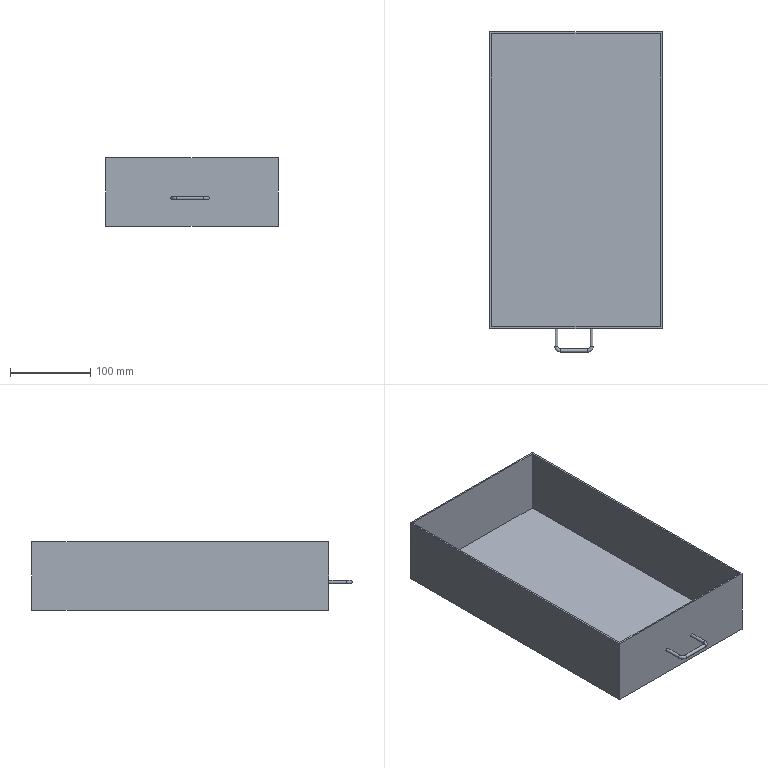Part | NX | features solid 2 | 1 solid | 16 faces | box 215 x 399 x 85 mm | volume 439303 mm3 | plane 11 | cylinder 3 | torus 2 | commonest cylinder face diameters 4 x3
STEP:
#1=CARTESIAN_POINT('',(143.,-305.,-247.));
#2=VERTEX_POINT('',#1);
#3=CARTESIAN_POINT('',(143.,-305.,-245.));
#4=DIRECTION('',(0.,-1.,0.));
#5=DIRECTION('',(0.,0.,-1.));
#6=AXIS2_PLACEMENT_3D('',#3,#4,#5);
#7=CIRCLE('',#6,2.);
#8=EDGE_CURVE('',#2,#2,#7,.F.);
#9=ORIENTED_EDGE('',*,*,#8,.T.);
#10=EDGE_LOOP('',(#9));
#11=FACE_BOUND('',#10,.T.);
#12=CARTESIAN_POINT('',(60.,-305.,-195.));
#13=VERTEX_POINT('',#12);
#14=CARTESIAN_POINT('',(275.,-305.,-195.));
#15=VERTEX_POINT('',#14);
#16=CARTESIAN_POINT('',(60.,-305.,-195.));
#17=DIRECTION('',(1.,0.,0.));
#18=VECTOR('',#17,1000.);
#19=LINE('',#16,#18);
#20=EDGE_CURVE('',#13,#15,#19,.T.);
#21=ORIENTED_EDGE('',*,*,#20,.F.);
#22=CARTESIAN_POINT('',(60.,-305.,-280.));
#23=VERTEX_POINT('',#22);
#24=CARTESIAN_POINT('',(60.,-305.,-145.));
#25=DIRECTION('',(0.,0.,-1.));
#26=VECTOR('',#25,1000.);
#27=LINE('',#24,#26);
#28=EDGE_CURVE('',#13,#23,#27,.T.);
#29=ORIENTED_EDGE('',*,*,#28,.T.);
#30=CARTESIAN_POINT('',(275.,-305.,-280.));
#31=VERTEX_POINT('',#30);
#32=CARTESIAN_POINT('',(60.,-305.,-280.));
#33=DIRECTION('',(1.,0.,0.));
#34=VECTOR('',#33,1000.);
#35=LINE('',#32,#34);
#36=EDGE_CURVE('',#23,#31,#35,.T.);
#37=ORIENTED_EDGE('',*,*,#36,.T.);
#38=CARTESIAN_POINT('',(275.,-305.,-145.));
#39=DIRECTION('',(0.,0.,-1.));
#40=VECTOR('',#39,1000.);
#41=LINE('',#38,#40);
#42=EDGE_CURVE('',#15,#31,#41,.T.);
#43=ORIENTED_EDGE('',*,*,#42,.F.);
#44=EDGE_LOOP('',(#21,#29,#37,#43));
#45=FACE_BOUND('',#44,.T.);
#46=CARTESIAN_POINT('',(187.,-305.,-243.));
#47=VERTEX_POINT('',#46);
#48=CARTESIAN_POINT('',(187.,-305.,-245.));
#49=DIRECTION('',(0.,1.,0.));
#50=DIRECTION('',(0.,0.,1.));
#51=AXIS2_PLACEMENT_3D('',#48,#49,#50);
#52=CIRCLE('',#51,2.);
#53=EDGE_CURVE('',#47,#47,#52,.F.);
#54=ORIENTED_EDGE('',*,*,#53,.F.);
#55=EDGE_LOOP('',(#54));
#56=FACE_BOUND('',#55,.T.);
#57=CARTESIAN_POINT('',(60.,-305.,-145.));
#58=DIRECTION('',(0.,1.,0.));
#59=DIRECTION('',(0.,0.,1.));
#60=AXIS2_PLACEMENT_3D('',#57,#58,#59);
#61=PLANE('',#60);
#62=ADVANCED_FACE('',(#11,#45,#56),#61,.F.);
#63=CARTESIAN_POINT('',(275.,65.,-195.));
#64=VERTEX_POINT('',#63);
#65=CARTESIAN_POINT('',(275.,-305.,-195.));
#66=DIRECTION('',(0.,1.,0.));
#67=VECTOR('',#66,1000.);
#68=LINE('',#65,#67);
#69=EDGE_CURVE('',#15,#64,#68,.T.);
#70=ORIENTED_EDGE('',*,*,#69,.F.);
#71=ORIENTED_EDGE('',*,*,#42,.T.);
#72=CARTESIAN_POINT('',(275.,65.,-280.));
#73=VERTEX_POINT('',#72);
#74=CARTESIAN_POINT('',(275.,-305.,-280.));
#75=DIRECTION('',(0.,1.,0.));
#76=VECTOR('',#75,1000.);
#77=LINE('',#74,#76);
#78=EDGE_CURVE('',#31,#73,#77,.T.);
#79=ORIENTED_EDGE('',*,*,#78,.T.);
#80=CARTESIAN_POINT('',(275.,65.,-145.));
#81=DIRECTION('',(0.,0.,-1.));
#82=VECTOR('',#81,1000.);
#83=LINE('',#80,#82);
#84=EDGE_CURVE('',#64,#73,#83,.T.);
#85=ORIENTED_EDGE('',*,*,#84,.F.);
#86=EDGE_LOOP('',(#70,#71,#79,#85));
#87=FACE_BOUND('',#86,.T.);
#88=CARTESIAN_POINT('',(275.,-305.,-145.));
#89=DIRECTION('',(-1.,0.,0.));
#90=DIRECTION('',(0.,0.,1.));
#91=AXIS2_PLACEMENT_3D('',#88,#89,#90);
#92=PLANE('',#91);
#93=ADVANCED_FACE('',(#87),#92,.F.);
#94=CARTESIAN_POINT('',(60.,65.,-195.));
#95=VERTEX_POINT('',#94);
#96=CARTESIAN_POINT('',(60.,-302.5,-195.));
#97=DIRECTION('',(0.,-1.,0.));
#98=VECTOR('',#97,1000.);
#99=LINE('',#96,#98);
#100=EDGE_CURVE('',#95,#13,#99,.T.);
#101=ORIENTED_EDGE('',*,*,#100,.F.);
#102=CARTESIAN_POINT('',(60.,65.,-280.));
#103=VERTEX_POINT('',#102);
#104=CARTESIAN_POINT('',(60.,65.,-145.));
#105=DIRECTION('',(0.,0.,-1.));
#106=VECTOR('',#105,1000.);
#107=LINE('',#104,#106);
#108=EDGE_CURVE('',#95,#103,#107,.T.);
#109=ORIENTED_EDGE('',*,*,#108,.T.);
#110=CARTESIAN_POINT('',(60.,-302.5,-280.));
#111=DIRECTION('',(0.,-1.,0.));
#112=VECTOR('',#111,1000.);
#113=LINE('',#110,#112);
#114=EDGE_CURVE('',#103,#23,#113,.T.);
#115=ORIENTED_EDGE('',*,*,#114,.T.);
#116=ORIENTED_EDGE('',*,*,#28,.F.);
#117=EDGE_LOOP('',(#101,#109,#115,#116));
#118=FACE_BOUND('',#117,.T.);
#119=CARTESIAN_POINT('',(60.,-302.5,-145.));
#120=DIRECTION('',(1.,0.,0.));
#121=DIRECTION('',(0.,0.,-1.));
#122=AXIS2_PLACEMENT_3D('',#119,#120,#121);
#123=PLANE('',#122);
#124=ADVANCED_FACE('',(#118),#123,.F.);
#125=CARTESIAN_POINT('',(280.,65.,-195.));
#126=DIRECTION('',(-1.,0.,0.));
#127=VECTOR('',#126,1000.);
#128=LINE('',#125,#127);
#129=EDGE_CURVE('',#64,#95,#128,.T.);
#130=ORIENTED_EDGE('',*,*,#129,.F.);
#131=ORIENTED_EDGE('',*,*,#84,.T.);
#132=CARTESIAN_POINT('',(280.,65.,-280.));
#133=DIRECTION('',(-1.,0.,0.));
#134=VECTOR('',#133,1000.);
#135=LINE('',#132,#134);
#136=EDGE_CURVE('',#73,#103,#135,.T.);
#137=ORIENTED_EDGE('',*,*,#136,.T.);
#138=ORIENTED_EDGE('',*,*,#108,.F.);
#139=EDGE_LOOP('',(#130,#131,#137,#138));
#140=FACE_BOUND('',#139,.T.);
#141=CARTESIAN_POINT('',(280.,65.,-145.));
#142=DIRECTION('',(0.,-1.,0.));
#143=DIRECTION('',(0.,0.,-1.));
#144=AXIS2_PLACEMENT_3D('',#141,#142,#143);
#145=PLANE('',#144);
#146=ADVANCED_FACE('',(#140),#145,.F.);
#147=ORIENTED_EDGE('',*,*,#136,.F.);
#148=ORIENTED_EDGE('',*,*,#78,.F.);
#149=ORIENTED_EDGE('',*,*,#36,.F.);
#150=ORIENTED_EDGE('',*,*,#114,.F.);
#151=EDGE_LOOP('',(#147,#148,#149,#150));
#152=FACE_BOUND('',#151,.T.);
#153=CARTESIAN_POINT('',(277.5,47.5,-280.));
#154=DIRECTION('',(0.,0.,1.));
#155=DIRECTION('',(1.,0.,0.));
#156=AXIS2_PLACEMENT_3D('',#153,#154,#155);
#157=PLANE('',#156);
#158=ADVANCED_FACE('',(#152),#157,.F.);
#159=CARTESIAN_POINT('',(272.5,-302.5,-195.));
#160=VERTEX_POINT('',#159);
#161=CARTESIAN_POINT('',(62.5,-302.5,-195.));
#162=VERTEX_POINT('',#161);
#163=CARTESIAN_POINT('',(280.,-302.5,-195.));
#164=DIRECTION('',(-1.,0.,0.));
#165=VECTOR('',#164,1000.);
#166=LINE('',#163,#165);
#167=EDGE_CURVE('',#160,#162,#166,.T.);
#168=ORIENTED_EDGE('',*,*,#167,.T.);
#169=CARTESIAN_POINT('',(62.5,62.5,-195.));
#170=VERTEX_POINT('',#169);
#171=CARTESIAN_POINT('',(62.5,-302.5,-195.));
#172=DIRECTION('',(0.,1.,0.));
#173=VECTOR('',#172,1000.);
#174=LINE('',#171,#173);
#175=EDGE_CURVE('',#162,#170,#174,.T.);
#176=ORIENTED_EDGE('',*,*,#175,.T.);
#177=CARTESIAN_POINT('',(272.5,62.5,-195.));
#178=VERTEX_POINT('',#177);
#179=CARTESIAN_POINT('',(60.,62.5,-195.));
#180=DIRECTION('',(1.,0.,0.));
#181=VECTOR('',#180,1000.);
#182=LINE('',#179,#181);
#183=EDGE_CURVE('',#170,#178,#182,.T.);
#184=ORIENTED_EDGE('',*,*,#183,.T.);
#185=CARTESIAN_POINT('',(272.5,47.5,-195.));
#186=DIRECTION('',(0.,-1.,0.));
#187=VECTOR('',#186,1000.);
#188=LINE('',#185,#187);
#189=EDGE_CURVE('',#178,#160,#188,.T.);
#190=ORIENTED_EDGE('',*,*,#189,.T.);
#191=EDGE_LOOP('',(#168,#176,#184,#190));
#192=FACE_BOUND('',#191,.T.);
#193=ORIENTED_EDGE('',*,*,#100,.T.);
#194=ORIENTED_EDGE('',*,*,#20,.T.);
#195=ORIENTED_EDGE('',*,*,#69,.T.);
#196=ORIENTED_EDGE('',*,*,#129,.T.);
#197=EDGE_LOOP('',(#193,#194,#195,#196));
#198=FACE_BOUND('',#197,.T.);
#199=CARTESIAN_POINT('',(0.,0.,-195.));
#200=DIRECTION('',(0.,0.,1.));
#201=DIRECTION('',(1.,0.,0.));
#202=AXIS2_PLACEMENT_3D('',#199,#200,#201);
#203=PLANE('',#202);
#204=ADVANCED_FACE('',(#192,#198),#203,.T.);
#205=CARTESIAN_POINT('',(272.5,-302.5,-277.5));
#206=VERTEX_POINT('',#205);
#207=CARTESIAN_POINT('',(272.5,62.5,-277.5));
#208=VERTEX_POINT('',#207);
#209=CARTESIAN_POINT('',(272.5,47.5,-277.5));
#210=DIRECTION('',(0.,1.,0.));
#211=VECTOR('',#210,1000.);
#212=LINE('',#209,#211);
#213=EDGE_CURVE('',#206,#208,#212,.T.);
#214=ORIENTED_EDGE('',*,*,#213,.T.);
#215=CARTESIAN_POINT('',(62.5,62.5,-277.5));
#216=VERTEX_POINT('',#215);
#217=CARTESIAN_POINT('',(277.5,62.5,-277.5));
#218=DIRECTION('',(-1.,0.,0.));
#219=VECTOR('',#218,1000.);
#220=LINE('',#217,#219);
#221=EDGE_CURVE('',#208,#216,#220,.T.);
#222=ORIENTED_EDGE('',*,*,#221,.T.);
#223=CARTESIAN_POINT('',(62.5,-302.5,-277.5));
#224=VERTEX_POINT('',#223);
#225=CARTESIAN_POINT('',(62.5,47.5,-277.5));
#226=DIRECTION('',(0.,-1.,0.));
#227=VECTOR('',#226,1000.);
#228=LINE('',#225,#227);
#229=EDGE_CURVE('',#216,#224,#228,.T.);
#230=ORIENTED_EDGE('',*,*,#229,.T.);
#231=CARTESIAN_POINT('',(62.5,-302.5,-277.5));
#232=DIRECTION('',(1.,0.,0.));
#233=VECTOR('',#232,1000.);
#234=LINE('',#231,#233);
#235=EDGE_CURVE('',#224,#206,#234,.T.);
#236=ORIENTED_EDGE('',*,*,#235,.T.);
#237=EDGE_LOOP('',(#214,#222,#230,#236));
#238=FACE_BOUND('',#237,.T.);
#239=CARTESIAN_POINT('',(277.5,47.5,-277.5));
#240=DIRECTION('',(0.,0.,1.));
#241=DIRECTION('',(1.,0.,0.));
#242=AXIS2_PLACEMENT_3D('',#239,#240,#241);
#243=PLANE('',#242);
#244=ADVANCED_FACE('',(#238),#243,.T.);
#245=ORIENTED_EDGE('',*,*,#189,.F.);
#246=CARTESIAN_POINT('',(272.5,62.5,-145.));
#247=DIRECTION('',(0.,0.,-1.));
#248=VECTOR('',#247,1000.);
#249=LINE('',#246,#248);
#250=EDGE_CURVE('',#178,#208,#249,.T.);
#251=ORIENTED_EDGE('',*,*,#250,.T.);
#252=ORIENTED_EDGE('',*,*,#213,.F.);
#253=CARTESIAN_POINT('',(272.5,-302.5,-145.));
#254=DIRECTION('',(0.,0.,-1.));
#255=VECTOR('',#254,1000.);
#256=LINE('',#253,#255);
#257=EDGE_CURVE('',#160,#206,#256,.T.);
#258=ORIENTED_EDGE('',*,*,#257,.F.);
#259=EDGE_LOOP('',(#245,#251,#252,#258));
#260=FACE_BOUND('',#259,.T.);
#261=CARTESIAN_POINT('',(272.5,47.5,-145.));
#262=DIRECTION('',(1.,0.,0.));
#263=DIRECTION('',(0.,0.,-1.));
#264=AXIS2_PLACEMENT_3D('',#261,#262,#263);
#265=PLANE('',#264);
#266=ADVANCED_FACE('',(#260),#265,.F.);
#267=ORIENTED_EDGE('',*,*,#175,.F.);
#268=CARTESIAN_POINT('',(62.5,-302.5,-145.));
#269=DIRECTION('',(0.,0.,-1.));
#270=VECTOR('',#269,1000.);
#271=LINE('',#268,#270);
#272=EDGE_CURVE('',#162,#224,#271,.T.);
#273=ORIENTED_EDGE('',*,*,#272,.T.);
#274=ORIENTED_EDGE('',*,*,#229,.F.);
#275=CARTESIAN_POINT('',(62.5,62.5,-145.));
#276=DIRECTION('',(0.,0.,-1.));
#277=VECTOR('',#276,1000.);
#278=LINE('',#275,#277);
#279=EDGE_CURVE('',#170,#216,#278,.T.);
#280=ORIENTED_EDGE('',*,*,#279,.F.);
#281=EDGE_LOOP('',(#267,#273,#274,#280));
#282=FACE_BOUND('',#281,.T.);
#283=CARTESIAN_POINT('',(62.5,-302.5,-145.));
#284=DIRECTION('',(-1.,0.,0.));
#285=DIRECTION('',(0.,0.,1.));
#286=AXIS2_PLACEMENT_3D('',#283,#284,#285);
#287=PLANE('',#286);
#288=ADVANCED_FACE('',(#282),#287,.F.);
#289=ORIENTED_EDGE('',*,*,#183,.F.);
#290=ORIENTED_EDGE('',*,*,#279,.T.);
#291=ORIENTED_EDGE('',*,*,#221,.F.);
#292=ORIENTED_EDGE('',*,*,#250,.F.);
#293=EDGE_LOOP('',(#289,#290,#291,#292));
#294=FACE_BOUND('',#293,.T.);
#295=CARTESIAN_POINT('',(60.,62.5,-145.));
#296=DIRECTION('',(0.,1.,0.));
#297=DIRECTION('',(0.,0.,1.));
#298=AXIS2_PLACEMENT_3D('',#295,#296,#297);
#299=PLANE('',#298);
#300=ADVANCED_FACE('',(#294),#299,.F.);
#301=ORIENTED_EDGE('',*,*,#167,.F.);
#302=ORIENTED_EDGE('',*,*,#257,.T.);
#303=ORIENTED_EDGE('',*,*,#235,.F.);
#304=ORIENTED_EDGE('',*,*,#272,.F.);
#305=EDGE_LOOP('',(#301,#302,#303,#304));
#306=FACE_BOUND('',#305,.T.);
#307=CARTESIAN_POINT('',(280.,-302.5,-145.));
#308=DIRECTION('',(0.,-1.,0.));
#309=DIRECTION('',(0.,0.,-1.));
#310=AXIS2_PLACEMENT_3D('',#307,#308,#309);
#311=PLANE('',#310);
#312=ADVANCED_FACE('',(#306),#311,.F.);
#313=CARTESIAN_POINT('',(148.,-332.,-247.));
#314=VERTEX_POINT('',#313);
#315=CARTESIAN_POINT('',(148.,-332.,-245.));
#316=DIRECTION('',(-1.,0.,0.));
#317=DIRECTION('',(0.,0.,-1.));
#318=AXIS2_PLACEMENT_3D('',#315,#316,#317);
#319=CIRCLE('',#318,2.);
#320=EDGE_CURVE('',#314,#314,#319,.T.);
#321=ORIENTED_EDGE('',*,*,#320,.T.);
#322=EDGE_LOOP('',(#321));
#323=FACE_BOUND('',#322,.T.);
#324=CARTESIAN_POINT('',(143.,-327.,-247.));
#325=VERTEX_POINT('',#324);
#326=CARTESIAN_POINT('',(143.,-327.,-245.));
#327=DIRECTION('',(0.,1.,0.));
#328=DIRECTION('',(0.,0.,-1.));
#329=AXIS2_PLACEMENT_3D('',#326,#327,#328);
#330=CIRCLE('',#329,2.);
#331=EDGE_CURVE('',#325,#325,#330,.T.);
#332=ORIENTED_EDGE('',*,*,#331,.F.);
#333=EDGE_LOOP('',(#332));
#334=FACE_BOUND('',#333,.T.);
#335=CARTESIAN_POINT('',(148.,-327.,-245.));
#336=DIRECTION('',(0.,0.,-1.));
#337=DIRECTION('',(-1.,0.,0.));
#338=AXIS2_PLACEMENT_3D('',#335,#336,#337);
#339=TOROIDAL_SURFACE('',#338,5.,2.);
#340=ADVANCED_FACE('',(#323,#334),#339,.T.);
#341=ORIENTED_EDGE('',*,*,#331,.T.);
#342=EDGE_LOOP('',(#341));
#343=FACE_BOUND('',#342,.T.);
#344=ORIENTED_EDGE('',*,*,#8,.F.);
#345=EDGE_LOOP('',(#344));
#346=FACE_BOUND('',#345,.T.);
#347=CARTESIAN_POINT('',(143.,-327.,-245.));
#348=DIRECTION('',(0.,1.,0.));
#349=DIRECTION('',(0.,0.,1.));
#350=AXIS2_PLACEMENT_3D('',#347,#348,#349);
#351=CYLINDRICAL_SURFACE('',#350,2.);
#352=ADVANCED_FACE('',(#343,#346),#351,.T.);
#353=CARTESIAN_POINT('',(182.,-332.,-247.));
#354=VERTEX_POINT('',#353);
#355=CARTESIAN_POINT('',(182.,-332.,-245.));
#356=DIRECTION('',(-1.,0.,0.));
#357=DIRECTION('',(0.,0.,-1.));
#358=AXIS2_PLACEMENT_3D('',#355,#356,#357);
#359=CIRCLE('',#358,2.);
#360=EDGE_CURVE('',#354,#354,#359,.T.);
#361=ORIENTED_EDGE('',*,*,#360,.T.);
#362=EDGE_LOOP('',(#361));
#363=FACE_BOUND('',#362,.T.);
#364=ORIENTED_EDGE('',*,*,#320,.F.);
#365=EDGE_LOOP('',(#364));
#366=FACE_BOUND('',#365,.T.);
#367=CARTESIAN_POINT('',(182.,-332.,-245.));
#368=DIRECTION('',(-1.,0.,0.));
#369=DIRECTION('',(0.,0.,1.));
#370=AXIS2_PLACEMENT_3D('',#367,#368,#369);
#371=CYLINDRICAL_SURFACE('',#370,2.);
#372=ADVANCED_FACE('',(#363,#366),#371,.T.);
#373=CARTESIAN_POINT('',(187.,-327.,-247.));
#374=VERTEX_POINT('',#373);
#375=CARTESIAN_POINT('',(187.,-327.,-245.));
#376=DIRECTION('',(0.,-1.,0.));
#377=DIRECTION('',(0.,0.,-1.));
#378=AXIS2_PLACEMENT_3D('',#375,#376,#377);
#379=CIRCLE('',#378,2.);
#380=EDGE_CURVE('',#374,#374,#379,.T.);
#381=ORIENTED_EDGE('',*,*,#380,.T.);
#382=EDGE_LOOP('',(#381));
#383=FACE_BOUND('',#382,.T.);
#384=ORIENTED_EDGE('',*,*,#360,.F.);
#385=EDGE_LOOP('',(#384));
#386=FACE_BOUND('',#385,.T.);
#387=CARTESIAN_POINT('',(182.,-327.,-245.));
#388=DIRECTION('',(0.,0.,-1.));
#389=DIRECTION('',(-1.,0.,0.));
#390=AXIS2_PLACEMENT_3D('',#387,#388,#389);
#391=TOROIDAL_SURFACE('',#390,5.,2.);
#392=ADVANCED_FACE('',(#383,#386),#391,.T.);
#393=ORIENTED_EDGE('',*,*,#380,.F.);
#394=EDGE_LOOP('',(#393));
#395=FACE_BOUND('',#394,.T.);
#396=ORIENTED_EDGE('',*,*,#53,.T.);
#397=EDGE_LOOP('',(#396));
#398=FACE_BOUND('',#397,.T.);
#399=CARTESIAN_POINT('',(187.,-327.,-245.));
#400=DIRECTION('',(0.,1.,0.));
#401=DIRECTION('',(0.,0.,1.));
#402=AXIS2_PLACEMENT_3D('',#399,#400,#401);
#403=CYLINDRICAL_SURFACE('',#402,2.);
#404=ADVANCED_FACE('',(#395,#398),#403,.T.);
#405=CLOSED_SHELL('',(#62,#93,#124,#146,#158,#204,#244,#266,#288,#300,#312,#340,#352,#372,#392,#404));
#406=MANIFOLD_SOLID_BREP('',#405);
#407=(LENGTH_UNIT()NAMED_UNIT(*)SI_UNIT(.MILLI.,.METRE.));
#408=UNCERTAINTY_MEASURE_WITH_UNIT(LENGTH_MEASURE(0.00001),#407,'','');
#409=(NAMED_UNIT(*)PLANE_ANGLE_UNIT()SI_UNIT($,.RADIAN.));
#410=(NAMED_UNIT(*)SI_UNIT($,.STERADIAN.)SOLID_ANGLE_UNIT());
#411=(GEOMETRIC_REPRESENTATION_CONTEXT(3)GLOBAL_UNCERTAINTY_ASSIGNED_CONTEXT((#408))GLOBAL_UNIT_ASSIGNED_CONTEXT((#407,#409,#410))REPRESENTATION_CONTEXT('',''));
#412=ADVANCED_BREP_SHAPE_REPRESENTATION('',(#406),#411);